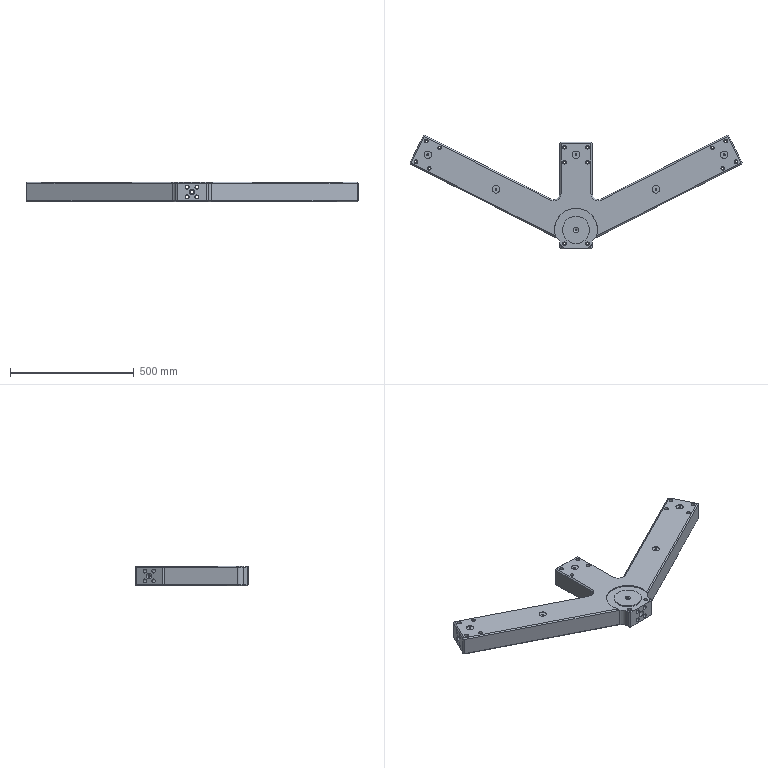Part | STEP file | solid 233 | 1 solid | 213 faces | box 1344 x 458.517 x 80 mm | volume 15931765 mm3 | cylinder 92 | plane 88 | cone 32 | sphere 1 | commonest cylinder face diameters 16 x18 9.4 x14 15 x14 12 x8 17 x6 5 x5